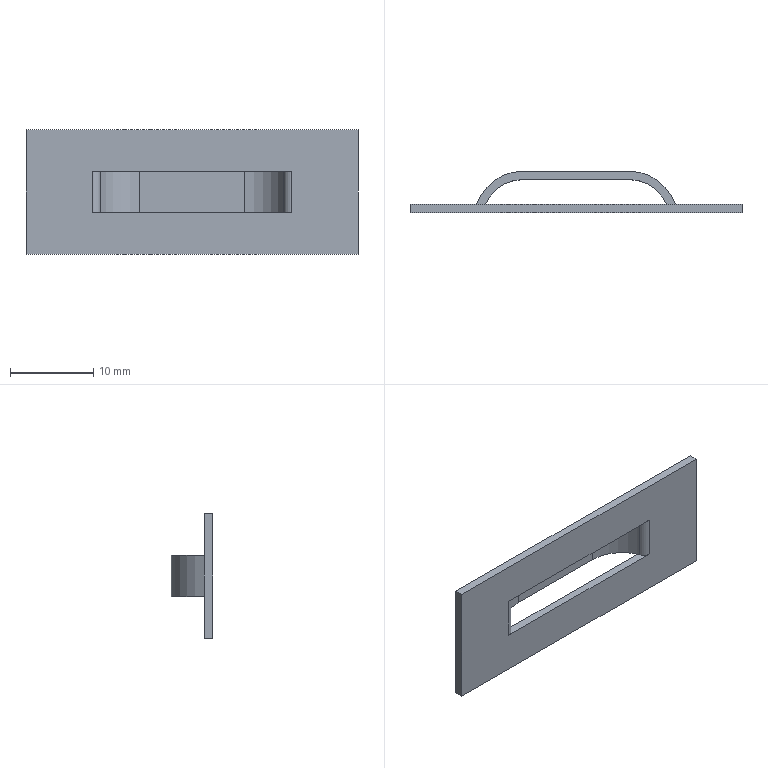Part | SolidWorks | features BaseBody 1 | 1 solid | 18 faces | box 40 x 5 x 15 mm | volume 617.289 mm3 | plane 12 | cylinder 6 | commonest cylinder face diameters 2 x2 10 x2 12 x2
STEP:
#1=CARTESIAN_POINT('',(-20.,0.,7.5));
#2=VERTEX_POINT('',#1);
#3=CARTESIAN_POINT('',(-20.,1.,7.5));
#4=VERTEX_POINT('',#3);
#5=CARTESIAN_POINT('',(-20.,-42.72,7.5));
#6=DIRECTION('',(0.,1.,0.));
#7=VECTOR('',#6,1000.);
#8=LINE('',#5,#7);
#9=EDGE_CURVE('',#2,#4,#8,.T.);
#10=ORIENTED_EDGE('',*,*,#9,.F.);
#11=CARTESIAN_POINT('',(20.,0.,7.5));
#12=VERTEX_POINT('',#11);
#13=CARTESIAN_POINT('',(20.,0.,7.5));
#14=DIRECTION('',(1.,0.,0.));
#15=VECTOR('',#14,1000.);
#16=LINE('',#13,#15);
#17=EDGE_CURVE('',#2,#12,#16,.T.);
#18=ORIENTED_EDGE('',*,*,#17,.T.);
#19=CARTESIAN_POINT('',(20.,1.,7.5));
#20=VERTEX_POINT('',#19);
#21=CARTESIAN_POINT('',(20.,-42.72,7.5));
#22=DIRECTION('',(0.,1.,0.));
#23=VECTOR('',#22,1000.);
#24=LINE('',#21,#23);
#25=EDGE_CURVE('',#12,#20,#24,.T.);
#26=ORIENTED_EDGE('',*,*,#25,.T.);
#27=CARTESIAN_POINT('',(20.,1.,7.5));
#28=DIRECTION('',(1.,0.,0.));
#29=VECTOR('',#28,1000.);
#30=LINE('',#27,#29);
#31=EDGE_CURVE('',#4,#20,#30,.T.);
#32=ORIENTED_EDGE('',*,*,#31,.F.);
#33=EDGE_LOOP('',(#10,#18,#26,#32));
#34=FACE_OUTER_BOUND('',#33,.T.);
#35=CARTESIAN_POINT('',(20.,-42.72,7.5));
#36=DIRECTION('',(0.,0.,1.));
#37=DIRECTION('',(1.,0.,0.));
#38=AXIS2_PLACEMENT_3D('',#35,#36,#37);
#39=PLANE('',#38);
#40=ADVANCED_FACE('',(#34),#39,.T.);
#41=CARTESIAN_POINT('',(-11.057,0.6667,2.5));
#42=VERTEX_POINT('',#41);
#43=CARTESIAN_POINT('',(-12.,0.,2.5));
#44=VERTEX_POINT('',#43);
#45=CARTESIAN_POINT('',(-12.,1.,2.5));
#46=DIRECTION('',(0.,0.,-1.));
#47=DIRECTION('',(1.,0.,0.));
#48=AXIS2_PLACEMENT_3D('',#45,#46,#47);
#49=CIRCLE('',#48,1.);
#50=EDGE_CURVE('',#42,#44,#49,.T.);
#51=ORIENTED_EDGE('',*,*,#50,.F.);
#52=CARTESIAN_POINT('',(-10.926,1.,2.5));
#53=VERTEX_POINT('',#52);
#54=CARTESIAN_POINT('',(-6.343,-1.,2.5));
#55=DIRECTION('',(0.,0.,1.));
#56=DIRECTION('',(-1.,0.,0.));
#57=AXIS2_PLACEMENT_3D('',#54,#55,#56);
#58=CIRCLE('',#57,5.);
#59=EDGE_CURVE('',#53,#42,#58,.T.);
#60=ORIENTED_EDGE('',*,*,#59,.F.);
#61=CARTESIAN_POINT('',(10.926,1.,2.5));
#62=VERTEX_POINT('',#61);
#63=CARTESIAN_POINT('',(12.,1.,2.5));
#64=DIRECTION('',(1.,0.,0.));
#65=VECTOR('',#64,1000.);
#66=LINE('',#63,#65);
#67=EDGE_CURVE('',#53,#62,#66,.T.);
#68=ORIENTED_EDGE('',*,*,#67,.T.);
#69=CARTESIAN_POINT('',(11.057,0.6667,2.5));
#70=VERTEX_POINT('',#69);
#71=CARTESIAN_POINT('',(6.343,-1.,2.5));
#72=DIRECTION('',(0.,0.,1.));
#73=DIRECTION('',(1.,0.,0.));
#74=AXIS2_PLACEMENT_3D('',#71,#72,#73);
#75=CIRCLE('',#74,5.);
#76=EDGE_CURVE('',#70,#62,#75,.T.);
#77=ORIENTED_EDGE('',*,*,#76,.F.);
#78=CARTESIAN_POINT('',(12.,0.,2.5));
#79=VERTEX_POINT('',#78);
#80=CARTESIAN_POINT('',(12.,1.,2.5));
#81=DIRECTION('',(0.,0.,-1.));
#82=DIRECTION('',(-1.,0.,0.));
#83=AXIS2_PLACEMENT_3D('',#80,#81,#82);
#84=CIRCLE('',#83,1.);
#85=EDGE_CURVE('',#79,#70,#84,.T.);
#86=ORIENTED_EDGE('',*,*,#85,.F.);
#87=CARTESIAN_POINT('',(12.,0.,2.5));
#88=DIRECTION('',(1.,0.,0.));
#89=VECTOR('',#88,1000.);
#90=LINE('',#87,#89);
#91=EDGE_CURVE('',#44,#79,#90,.T.);
#92=ORIENTED_EDGE('',*,*,#91,.F.);
#93=EDGE_LOOP('',(#51,#60,#68,#77,#86,#92));
#94=FACE_OUTER_BOUND('',#93,.T.);
#95=CARTESIAN_POINT('',(12.,-42.72,2.5));
#96=DIRECTION('',(0.,0.,1.));
#97=DIRECTION('',(1.,0.,0.));
#98=AXIS2_PLACEMENT_3D('',#95,#96,#97);
#99=PLANE('',#98);
#100=ADVANCED_FACE('',(#94),#99,.F.);
#101=CARTESIAN_POINT('',(-11.057,0.6667,-2.5));
#102=VERTEX_POINT('',#101);
#103=CARTESIAN_POINT('',(-12.,0.,-2.5));
#104=VERTEX_POINT('',#103);
#105=CARTESIAN_POINT('',(-12.,1.,-2.5));
#106=DIRECTION('',(0.,0.,-1.));
#107=DIRECTION('',(1.,0.,0.));
#108=AXIS2_PLACEMENT_3D('',#105,#106,#107);
#109=CIRCLE('',#108,1.);
#110=EDGE_CURVE('',#102,#104,#109,.T.);
#111=ORIENTED_EDGE('',*,*,#110,.T.);
#112=CARTESIAN_POINT('',(12.,0.,-2.5));
#113=VERTEX_POINT('',#112);
#114=CARTESIAN_POINT('',(-12.,0.,-2.5));
#115=DIRECTION('',(-1.,0.,0.));
#116=VECTOR('',#115,1000.);
#117=LINE('',#114,#116);
#118=EDGE_CURVE('',#113,#104,#117,.T.);
#119=ORIENTED_EDGE('',*,*,#118,.F.);
#120=CARTESIAN_POINT('',(11.057,0.6667,-2.5));
#121=VERTEX_POINT('',#120);
#122=CARTESIAN_POINT('',(12.,1.,-2.5));
#123=DIRECTION('',(0.,0.,-1.));
#124=DIRECTION('',(-1.,0.,0.));
#125=AXIS2_PLACEMENT_3D('',#122,#123,#124);
#126=CIRCLE('',#125,1.);
#127=EDGE_CURVE('',#113,#121,#126,.T.);
#128=ORIENTED_EDGE('',*,*,#127,.T.);
#129=CARTESIAN_POINT('',(10.926,1.,-2.5));
#130=VERTEX_POINT('',#129);
#131=CARTESIAN_POINT('',(6.343,-1.,-2.5));
#132=DIRECTION('',(0.,0.,1.));
#133=DIRECTION('',(1.,0.,0.));
#134=AXIS2_PLACEMENT_3D('',#131,#132,#133);
#135=CIRCLE('',#134,5.);
#136=EDGE_CURVE('',#121,#130,#135,.T.);
#137=ORIENTED_EDGE('',*,*,#136,.T.);
#138=CARTESIAN_POINT('',(-10.926,1.,-2.5));
#139=VERTEX_POINT('',#138);
#140=CARTESIAN_POINT('',(-12.,1.,-2.5));
#141=DIRECTION('',(-1.,0.,0.));
#142=VECTOR('',#141,1000.);
#143=LINE('',#140,#142);
#144=EDGE_CURVE('',#130,#139,#143,.T.);
#145=ORIENTED_EDGE('',*,*,#144,.T.);
#146=CARTESIAN_POINT('',(-6.343,-1.,-2.5));
#147=DIRECTION('',(0.,0.,1.));
#148=DIRECTION('',(-1.,0.,0.));
#149=AXIS2_PLACEMENT_3D('',#146,#147,#148);
#150=CIRCLE('',#149,5.);
#151=EDGE_CURVE('',#139,#102,#150,.T.);
#152=ORIENTED_EDGE('',*,*,#151,.T.);
#153=EDGE_LOOP('',(#111,#119,#128,#137,#145,#152));
#154=FACE_OUTER_BOUND('',#153,.T.);
#155=CARTESIAN_POINT('',(-12.,-42.72,-2.5));
#156=DIRECTION('',(0.,0.,-1.));
#157=DIRECTION('',(0.,-1.,0.));
#158=AXIS2_PLACEMENT_3D('',#155,#156,#157);
#159=PLANE('',#158);
#160=ADVANCED_FACE('',(#154),#159,.F.);
#161=CARTESIAN_POINT('',(20.,0.,-7.5));
#162=VERTEX_POINT('',#161);
#163=CARTESIAN_POINT('',(20.,1.,-7.5));
#164=VERTEX_POINT('',#163);
#165=CARTESIAN_POINT('',(20.,-42.72,-7.5));
#166=DIRECTION('',(0.,1.,0.));
#167=VECTOR('',#166,1000.);
#168=LINE('',#165,#167);
#169=EDGE_CURVE('',#162,#164,#168,.T.);
#170=ORIENTED_EDGE('',*,*,#169,.F.);
#171=CARTESIAN_POINT('',(-20.,0.,-7.5));
#172=VERTEX_POINT('',#171);
#173=CARTESIAN_POINT('',(20.,0.,-7.5));
#174=DIRECTION('',(-1.,0.,0.));
#175=VECTOR('',#174,1000.);
#176=LINE('',#173,#175);
#177=EDGE_CURVE('',#162,#172,#176,.T.);
#178=ORIENTED_EDGE('',*,*,#177,.T.);
#179=CARTESIAN_POINT('',(-20.,1.,-7.5));
#180=VERTEX_POINT('',#179);
#181=CARTESIAN_POINT('',(-20.,-42.72,-7.5));
#182=DIRECTION('',(0.,1.,0.));
#183=VECTOR('',#182,1000.);
#184=LINE('',#181,#183);
#185=EDGE_CURVE('',#172,#180,#184,.T.);
#186=ORIENTED_EDGE('',*,*,#185,.T.);
#187=CARTESIAN_POINT('',(20.,1.,-7.5));
#188=DIRECTION('',(-1.,0.,0.));
#189=VECTOR('',#188,1000.);
#190=LINE('',#187,#189);
#191=EDGE_CURVE('',#164,#180,#190,.T.);
#192=ORIENTED_EDGE('',*,*,#191,.F.);
#193=EDGE_LOOP('',(#170,#178,#186,#192));
#194=FACE_OUTER_BOUND('',#193,.T.);
#195=CARTESIAN_POINT('',(20.,-42.72,-7.5));
#196=DIRECTION('',(0.,0.,-1.));
#197=DIRECTION('',(0.,-1.,0.));
#198=AXIS2_PLACEMENT_3D('',#195,#196,#197);
#199=PLANE('',#198);
#200=ADVANCED_FACE('',(#194),#199,.T.);
#201=CARTESIAN_POINT('',(-6.343,5.,-2.5));
#202=VERTEX_POINT('',#201);
#203=CARTESIAN_POINT('',(-12.,1.,-2.5));
#204=VERTEX_POINT('',#203);
#205=CARTESIAN_POINT('',(-6.343,-1.,-2.5));
#206=DIRECTION('',(0.,0.,1.));
#207=DIRECTION('',(1.,0.,0.));
#208=AXIS2_PLACEMENT_3D('',#205,#206,#207);
#209=CIRCLE('',#208,6.);
#210=EDGE_CURVE('',#202,#204,#209,.T.);
#211=ORIENTED_EDGE('',*,*,#210,.T.);
#212=CARTESIAN_POINT('',(-12.,1.,2.5));
#213=VERTEX_POINT('',#212);
#214=CARTESIAN_POINT('',(-12.,1.,2.5));
#215=DIRECTION('',(0.,0.,-1.));
#216=VECTOR('',#215,1000.);
#217=LINE('',#214,#216);
#218=EDGE_CURVE('',#213,#204,#217,.T.);
#219=ORIENTED_EDGE('',*,*,#218,.F.);
#220=CARTESIAN_POINT('',(-6.343,5.,2.5));
#221=VERTEX_POINT('',#220);
#222=CARTESIAN_POINT('',(-6.343,-1.,2.5));
#223=DIRECTION('',(0.,0.,1.));
#224=DIRECTION('',(1.,0.,0.));
#225=AXIS2_PLACEMENT_3D('',#222,#223,#224);
#226=CIRCLE('',#225,6.);
#227=EDGE_CURVE('',#221,#213,#226,.T.);
#228=ORIENTED_EDGE('',*,*,#227,.F.);
#229=CARTESIAN_POINT('',(-6.343,5.,2.5));
#230=DIRECTION('',(0.,0.,-1.));
#231=VECTOR('',#230,1000.);
#232=LINE('',#229,#231);
#233=EDGE_CURVE('',#221,#202,#232,.T.);
#234=ORIENTED_EDGE('',*,*,#233,.T.);
#235=EDGE_LOOP('',(#211,#219,#228,#234));
#236=FACE_OUTER_BOUND('',#235,.T.);
#237=CARTESIAN_POINT('',(-6.343,-1.,2.5));
#238=DIRECTION('',(0.,0.,-1.));
#239=DIRECTION('',(-1.,0.,0.));
#240=AXIS2_PLACEMENT_3D('',#237,#238,#239);
#241=CYLINDRICAL_SURFACE('',#240,6.);
#242=ADVANCED_FACE('',(#236),#241,.T.);
#243=CARTESIAN_POINT('',(6.343,5.,-2.5));
#244=VERTEX_POINT('',#243);
#245=CARTESIAN_POINT('',(-6.343,5.,-2.5));
#246=DIRECTION('',(-1.,0.,0.));
#247=VECTOR('',#246,1000.);
#248=LINE('',#245,#247);
#249=EDGE_CURVE('',#244,#202,#248,.T.);
#250=ORIENTED_EDGE('',*,*,#249,.T.);
#251=ORIENTED_EDGE('',*,*,#233,.F.);
#252=CARTESIAN_POINT('',(6.343,5.,2.5));
#253=VERTEX_POINT('',#252);
#254=CARTESIAN_POINT('',(-6.343,5.,2.5));
#255=DIRECTION('',(-1.,0.,0.));
#256=VECTOR('',#255,1000.);
#257=LINE('',#254,#256);
#258=EDGE_CURVE('',#253,#221,#257,.T.);
#259=ORIENTED_EDGE('',*,*,#258,.F.);
#260=CARTESIAN_POINT('',(6.343,5.,2.5));
#261=DIRECTION('',(0.,0.,-1.));
#262=VECTOR('',#261,1000.);
#263=LINE('',#260,#262);
#264=EDGE_CURVE('',#253,#244,#263,.T.);
#265=ORIENTED_EDGE('',*,*,#264,.T.);
#266=EDGE_LOOP('',(#250,#251,#259,#265));
#267=FACE_OUTER_BOUND('',#266,.T.);
#268=CARTESIAN_POINT('',(-6.343,5.,2.5));
#269=DIRECTION('',(0.,-1.,0.));
#270=DIRECTION('',(0.,0.,-1.));
#271=AXIS2_PLACEMENT_3D('',#268,#269,#270);
#272=PLANE('',#271);
#273=ADVANCED_FACE('',(#267),#272,.F.);
#274=CARTESIAN_POINT('',(12.,1.,-2.5));
#275=VERTEX_POINT('',#274);
#276=CARTESIAN_POINT('',(6.343,-1.,-2.5));
#277=DIRECTION('',(0.,0.,1.));
#278=DIRECTION('',(1.,0.,0.));
#279=AXIS2_PLACEMENT_3D('',#276,#277,#278);
#280=CIRCLE('',#279,6.);
#281=EDGE_CURVE('',#275,#244,#280,.T.);
#282=ORIENTED_EDGE('',*,*,#281,.T.);
#283=ORIENTED_EDGE('',*,*,#264,.F.);
#284=CARTESIAN_POINT('',(12.,1.,2.5));
#285=VERTEX_POINT('',#284);
#286=CARTESIAN_POINT('',(6.343,-1.,2.5));
#287=DIRECTION('',(0.,0.,1.));
#288=DIRECTION('',(1.,0.,0.));
#289=AXIS2_PLACEMENT_3D('',#286,#287,#288);
#290=CIRCLE('',#289,6.);
#291=EDGE_CURVE('',#285,#253,#290,.T.);
#292=ORIENTED_EDGE('',*,*,#291,.F.);
#293=CARTESIAN_POINT('',(12.,1.,2.5));
#294=DIRECTION('',(0.,0.,-1.));
#295=VECTOR('',#294,1000.);
#296=LINE('',#293,#295);
#297=EDGE_CURVE('',#285,#275,#296,.T.);
#298=ORIENTED_EDGE('',*,*,#297,.T.);
#299=EDGE_LOOP('',(#282,#283,#292,#298));
#300=FACE_OUTER_BOUND('',#299,.T.);
#301=CARTESIAN_POINT('',(6.343,-1.,2.5));
#302=DIRECTION('',(0.,0.,-1.));
#303=DIRECTION('',(-1.,0.,0.));
#304=AXIS2_PLACEMENT_3D('',#301,#302,#303);
#305=CYLINDRICAL_SURFACE('',#304,6.);
#306=ADVANCED_FACE('',(#300),#305,.T.);
#307=ORIENTED_EDGE('',*,*,#297,.F.);
#308=CARTESIAN_POINT('',(12.,1.,2.5));
#309=DIRECTION('',(1.,0.,0.));
#310=VECTOR('',#309,1000.);
#311=LINE('',#308,#310);
#312=EDGE_CURVE('',#62,#285,#311,.T.);
#313=ORIENTED_EDGE('',*,*,#312,.F.);
#314=ORIENTED_EDGE('',*,*,#67,.F.);
#315=CARTESIAN_POINT('',(12.,1.,2.5));
#316=DIRECTION('',(1.,0.,0.));
#317=VECTOR('',#316,1000.);
#318=LINE('',#315,#317);
#319=EDGE_CURVE('',#213,#53,#318,.T.);
#320=ORIENTED_EDGE('',*,*,#319,.F.);
#321=ORIENTED_EDGE('',*,*,#218,.T.);
#322=CARTESIAN_POINT('',(-12.,1.,-2.5));
#323=DIRECTION('',(-1.,0.,0.));
#324=VECTOR('',#323,1000.);
#325=LINE('',#322,#324);
#326=EDGE_CURVE('',#139,#204,#325,.T.);
#327=ORIENTED_EDGE('',*,*,#326,.F.);
#328=ORIENTED_EDGE('',*,*,#144,.F.);
#329=CARTESIAN_POINT('',(-12.,1.,-2.5));
#330=DIRECTION('',(-1.,0.,0.));
#331=VECTOR('',#330,1000.);
#332=LINE('',#329,#331);
#333=EDGE_CURVE('',#275,#130,#332,.T.);
#334=ORIENTED_EDGE('',*,*,#333,.F.);
#335=EDGE_LOOP('',(#307,#313,#314,#320,#321,#327,#328,#334));
#336=FACE_BOUND('',#335,.T.);
#337=CARTESIAN_POINT('',(20.,1.,2.5));
#338=DIRECTION('',(0.,0.,-1.));
#339=VECTOR('',#338,1000.);
#340=LINE('',#337,#339);
#341=EDGE_CURVE('',#20,#164,#340,.T.);
#342=ORIENTED_EDGE('',*,*,#341,.T.);
#343=ORIENTED_EDGE('',*,*,#191,.T.);
#344=CARTESIAN_POINT('',(-20.,1.,2.5));
#345=DIRECTION('',(0.,0.,-1.));
#346=VECTOR('',#345,1000.);
#347=LINE('',#344,#346);
#348=EDGE_CURVE('',#4,#180,#347,.T.);
#349=ORIENTED_EDGE('',*,*,#348,.F.);
#350=ORIENTED_EDGE('',*,*,#31,.T.);
#351=EDGE_LOOP('',(#342,#343,#349,#350));
#352=FACE_OUTER_BOUND('',#351,.T.);
#353=CARTESIAN_POINT('',(20.,1.,2.5));
#354=DIRECTION('',(0.,-1.,0.));
#355=DIRECTION('',(-1.,0.,0.));
#356=AXIS2_PLACEMENT_3D('',#353,#354,#355);
#357=PLANE('',#356);
#358=ADVANCED_FACE('',(#336,#352),#357,.F.);
#359=CARTESIAN_POINT('',(20.,0.,2.5));
#360=DIRECTION('',(0.,0.,-1.));
#361=VECTOR('',#360,1000.);
#362=LINE('',#359,#361);
#363=EDGE_CURVE('',#12,#162,#362,.T.);
#364=ORIENTED_EDGE('',*,*,#363,.T.);
#365=ORIENTED_EDGE('',*,*,#169,.T.);
#366=ORIENTED_EDGE('',*,*,#341,.F.);
#367=ORIENTED_EDGE('',*,*,#25,.F.);
#368=EDGE_LOOP('',(#364,#365,#366,#367));
#369=FACE_OUTER_BOUND('',#368,.T.);
#370=CARTESIAN_POINT('',(20.,1.,2.5));
#371=DIRECTION('',(1.,0.,0.));
#372=DIRECTION('',(0.,1.,0.));
#373=AXIS2_PLACEMENT_3D('',#370,#371,#372);
#374=PLANE('',#373);
#375=ADVANCED_FACE('',(#369),#374,.T.);
#376=ORIENTED_EDGE('',*,*,#91,.T.);
#377=CARTESIAN_POINT('',(12.,0.,2.5));
#378=DIRECTION('',(0.,0.,-1.));
#379=VECTOR('',#378,1000.);
#380=LINE('',#377,#379);
#381=EDGE_CURVE('',#79,#113,#380,.T.);
#382=ORIENTED_EDGE('',*,*,#381,.T.);
#383=ORIENTED_EDGE('',*,*,#118,.T.);
#384=CARTESIAN_POINT('',(-12.,0.,2.5));
#385=DIRECTION('',(0.,0.,-1.));
#386=VECTOR('',#385,1000.);
#387=LINE('',#384,#386);
#388=EDGE_CURVE('',#44,#104,#387,.T.);
#389=ORIENTED_EDGE('',*,*,#388,.F.);
#390=EDGE_LOOP('',(#376,#382,#383,#389));
#391=FACE_BOUND('',#390,.T.);
#392=ORIENTED_EDGE('',*,*,#363,.F.);
#393=ORIENTED_EDGE('',*,*,#17,.F.);
#394=CARTESIAN_POINT('',(-20.,0.,2.5));
#395=DIRECTION('',(0.,0.,-1.));
#396=VECTOR('',#395,1000.);
#397=LINE('',#394,#396);
#398=EDGE_CURVE('',#2,#172,#397,.T.);
#399=ORIENTED_EDGE('',*,*,#398,.T.);
#400=ORIENTED_EDGE('',*,*,#177,.F.);
#401=EDGE_LOOP('',(#392,#393,#399,#400));
#402=FACE_OUTER_BOUND('',#401,.T.);
#403=CARTESIAN_POINT('',(20.,0.,2.5));
#404=DIRECTION('',(0.,-1.,0.));
#405=DIRECTION('',(-1.,0.,0.));
#406=AXIS2_PLACEMENT_3D('',#403,#404,#405);
#407=PLANE('',#406);
#408=ADVANCED_FACE('',(#391,#402),#407,.T.);
#409=ORIENTED_EDGE('',*,*,#127,.F.);
#410=ORIENTED_EDGE('',*,*,#381,.F.);
#411=ORIENTED_EDGE('',*,*,#85,.T.);
#412=CARTESIAN_POINT('',(11.057,0.6667,2.5));
#413=DIRECTION('',(0.,0.,-1.));
#414=VECTOR('',#413,1000.);
#415=LINE('',#412,#414);
#416=EDGE_CURVE('',#70,#121,#415,.T.);
#417=ORIENTED_EDGE('',*,*,#416,.T.);
#418=EDGE_LOOP('',(#409,#410,#411,#417));
#419=FACE_OUTER_BOUND('',#418,.T.);
#420=CARTESIAN_POINT('',(12.,1.,2.5));
#421=DIRECTION('',(0.,0.,-1.));
#422=DIRECTION('',(-1.,0.,0.));
#423=AXIS2_PLACEMENT_3D('',#420,#421,#422);
#424=CYLINDRICAL_SURFACE('',#423,1.);
#425=ADVANCED_FACE('',(#419),#424,.T.);
#426=ORIENTED_EDGE('',*,*,#136,.F.);
#427=ORIENTED_EDGE('',*,*,#416,.F.);
#428=ORIENTED_EDGE('',*,*,#76,.T.);
#429=CARTESIAN_POINT('',(6.343,4.,2.5));
#430=VERTEX_POINT('',#429);
#431=CARTESIAN_POINT('',(6.343,-1.,2.5));
#432=DIRECTION('',(0.,0.,1.));
#433=DIRECTION('',(1.,0.,0.));
#434=AXIS2_PLACEMENT_3D('',#431,#432,#433);
#435=CIRCLE('',#434,5.);
#436=EDGE_CURVE('',#62,#430,#435,.T.);
#437=ORIENTED_EDGE('',*,*,#436,.T.);
#438=CARTESIAN_POINT('',(6.343,4.,-2.5));
#439=VERTEX_POINT('',#438);
#440=CARTESIAN_POINT('',(6.343,4.,2.5));
#441=DIRECTION('',(0.,0.,-1.));
#442=VECTOR('',#441,1000.);
#443=LINE('',#440,#442);
#444=EDGE_CURVE('',#430,#439,#443,.T.);
#445=ORIENTED_EDGE('',*,*,#444,.T.);
#446=CARTESIAN_POINT('',(6.343,-1.,-2.5));
#447=DIRECTION('',(0.,0.,1.));
#448=DIRECTION('',(1.,0.,0.));
#449=AXIS2_PLACEMENT_3D('',#446,#447,#448);
#450=CIRCLE('',#449,5.);
#451=EDGE_CURVE('',#130,#439,#450,.T.);
#452=ORIENTED_EDGE('',*,*,#451,.F.);
#453=EDGE_LOOP('',(#426,#427,#428,#437,#445,#452));
#454=FACE_OUTER_BOUND('',#453,.T.);
#455=CARTESIAN_POINT('',(6.343,-1.,2.5));
#456=DIRECTION('',(0.,0.,-1.));
#457=DIRECTION('',(-1.,0.,0.));
#458=AXIS2_PLACEMENT_3D('',#455,#456,#457);
#459=CYLINDRICAL_SURFACE('',#458,5.);
#460=ADVANCED_FACE('',(#454),#459,.F.);
#461=CARTESIAN_POINT('',(-6.343,4.,-2.5));
#462=VERTEX_POINT('',#461);
#463=CARTESIAN_POINT('',(-6.343,4.,-2.5));
#464=DIRECTION('',(-1.,0.,0.));
#465=VECTOR('',#464,1000.);
#466=LINE('',#463,#465);
#467=EDGE_CURVE('',#439,#462,#466,.T.);
#468=ORIENTED_EDGE('',*,*,#467,.F.);
#469=ORIENTED_EDGE('',*,*,#444,.F.);
#470=CARTESIAN_POINT('',(-6.343,4.,2.5));
#471=VERTEX_POINT('',#470);
#472=CARTESIAN_POINT('',(-6.343,4.,2.5));
#473=DIRECTION('',(-1.,0.,0.));
#474=VECTOR('',#473,1000.);
#475=LINE('',#472,#474);
#476=EDGE_CURVE('',#430,#471,#475,.T.);
#477=ORIENTED_EDGE('',*,*,#476,.T.);
#478=CARTESIAN_POINT('',(-6.343,4.,2.5));
#479=DIRECTION('',(0.,0.,-1.));
#480=VECTOR('',#479,1000.);
#481=LINE('',#478,#480);
#482=EDGE_CURVE('',#471,#462,#481,.T.);
#483=ORIENTED_EDGE('',*,*,#482,.T.);
#484=EDGE_LOOP('',(#468,#469,#477,#483));
#485=FACE_OUTER_BOUND('',#484,.T.);
#486=CARTESIAN_POINT('',(-6.343,4.,2.5));
#487=DIRECTION('',(0.,-1.,0.));
#488=DIRECTION('',(0.,0.,-1.));
#489=AXIS2_PLACEMENT_3D('',#486,#487,#488);
#490=PLANE('',#489);
#491=ADVANCED_FACE('',(#485),#490,.T.);
#492=CARTESIAN_POINT('',(-6.343,-1.,-2.5));
#493=DIRECTION('',(0.,0.,1.));
#494=DIRECTION('',(-1.,0.,0.));
#495=AXIS2_PLACEMENT_3D('',#492,#493,#494);
#496=CIRCLE('',#495,5.);
#497=EDGE_CURVE('',#462,#139,#496,.T.);
#498=ORIENTED_EDGE('',*,*,#497,.F.);
#499=ORIENTED_EDGE('',*,*,#482,.F.);
#500=CARTESIAN_POINT('',(-6.343,-1.,2.5));
#501=DIRECTION('',(0.,0.,1.));
#502=DIRECTION('',(-1.,0.,0.));
#503=AXIS2_PLACEMENT_3D('',#500,#501,#502);
#504=CIRCLE('',#503,5.);
#505=EDGE_CURVE('',#471,#53,#504,.T.);
#506=ORIENTED_EDGE('',*,*,#505,.T.);
#507=ORIENTED_EDGE('',*,*,#59,.T.);
#508=CARTESIAN_POINT('',(-11.057,0.6667,2.5));
#509=DIRECTION('',(0.,0.,-1.));
#510=VECTOR('',#509,1000.);
#511=LINE('',#508,#510);
#512=EDGE_CURVE('',#42,#102,#511,.T.);
#513=ORIENTED_EDGE('',*,*,#512,.T.);
#514=ORIENTED_EDGE('',*,*,#151,.F.);
#515=EDGE_LOOP('',(#498,#499,#506,#507,#513,#514));
#516=FACE_OUTER_BOUND('',#515,.T.);
#517=CARTESIAN_POINT('',(-6.343,-1.,2.5));
#518=DIRECTION('',(0.,0.,-1.));
#519=DIRECTION('',(-1.,0.,0.));
#520=AXIS2_PLACEMENT_3D('',#517,#518,#519);
#521=CYLINDRICAL_SURFACE('',#520,5.);
#522=ADVANCED_FACE('',(#516),#521,.F.);
#523=ORIENTED_EDGE('',*,*,#110,.F.);
#524=ORIENTED_EDGE('',*,*,#512,.F.);
#525=ORIENTED_EDGE('',*,*,#50,.T.);
#526=ORIENTED_EDGE('',*,*,#388,.T.);
#527=EDGE_LOOP('',(#523,#524,#525,#526));
#528=FACE_OUTER_BOUND('',#527,.T.);
#529=CARTESIAN_POINT('',(-12.,1.,2.5));
#530=DIRECTION('',(0.,0.,-1.));
#531=DIRECTION('',(-1.,0.,0.));
#532=AXIS2_PLACEMENT_3D('',#529,#530,#531);
#533=CYLINDRICAL_SURFACE('',#532,1.);
#534=ADVANCED_FACE('',(#528),#533,.T.);
#535=ORIENTED_EDGE('',*,*,#348,.T.);
#536=ORIENTED_EDGE('',*,*,#185,.F.);
#537=ORIENTED_EDGE('',*,*,#398,.F.);
#538=ORIENTED_EDGE('',*,*,#9,.T.);
#539=EDGE_LOOP('',(#535,#536,#537,#538));
#540=FACE_OUTER_BOUND('',#539,.T.);
#541=CARTESIAN_POINT('',(-20.,0.,2.5));
#542=DIRECTION('',(-1.,0.,0.));
#543=DIRECTION('',(0.,0.,1.));
#544=AXIS2_PLACEMENT_3D('',#541,#542,#543);
#545=PLANE('',#544);
#546=ADVANCED_FACE('',(#540),#545,.T.);
#547=ORIENTED_EDGE('',*,*,#281,.F.);
#548=ORIENTED_EDGE('',*,*,#333,.T.);
#549=ORIENTED_EDGE('',*,*,#451,.T.);
#550=ORIENTED_EDGE('',*,*,#467,.T.);
#551=ORIENTED_EDGE('',*,*,#497,.T.);
#552=ORIENTED_EDGE('',*,*,#326,.T.);
#553=ORIENTED_EDGE('',*,*,#210,.F.);
#554=ORIENTED_EDGE('',*,*,#249,.F.);
#555=EDGE_LOOP('',(#547,#548,#549,#550,#551,#552,#553,#554));
#556=FACE_OUTER_BOUND('',#555,.T.);
#557=CARTESIAN_POINT('',(-12.,1.,-2.5));
#558=DIRECTION('',(0.,0.,-1.));
#559=DIRECTION('',(0.,-1.,0.));
#560=AXIS2_PLACEMENT_3D('',#557,#558,#559);
#561=PLANE('',#560);
#562=ADVANCED_FACE('',(#556),#561,.T.);
#563=ORIENTED_EDGE('',*,*,#312,.T.);
#564=ORIENTED_EDGE('',*,*,#291,.T.);
#565=ORIENTED_EDGE('',*,*,#258,.T.);
#566=ORIENTED_EDGE('',*,*,#227,.T.);
#567=ORIENTED_EDGE('',*,*,#319,.T.);
#568=ORIENTED_EDGE('',*,*,#505,.F.);
#569=ORIENTED_EDGE('',*,*,#476,.F.);
#570=ORIENTED_EDGE('',*,*,#436,.F.);
#571=EDGE_LOOP('',(#563,#564,#565,#566,#567,#568,#569,#570));
#572=FACE_OUTER_BOUND('',#571,.T.);
#573=CARTESIAN_POINT('',(-12.,1.,2.5));
#574=DIRECTION('',(0.,0.,-1.));
#575=DIRECTION('',(0.,-1.,0.));
#576=AXIS2_PLACEMENT_3D('',#573,#574,#575);
#577=PLANE('',#576);
#578=ADVANCED_FACE('',(#572),#577,.F.);
#579=CLOSED_SHELL('',(#40,#100,#160,#200,#242,#273,#306,#358,#375,#408,#425,#460,#491,#522,#534,#546,#562,#578));
#580=MANIFOLD_SOLID_BREP('',#579);
#581=CARTESIAN_POINT('',(0.,0.,0.));
#582=DIRECTION('',(0.,0.,1.));
#583=DIRECTION('',(1.,0.,0.));
#584=AXIS2_PLACEMENT_3D('',#581,#582,#583);
#585=(LENGTH_UNIT()NAMED_UNIT(*)SI_UNIT(.MILLI.,.METRE.));
#586=UNCERTAINTY_MEASURE_WITH_UNIT(LENGTH_MEASURE(0.00001),#585,'','');
#587=(NAMED_UNIT(*)PLANE_ANGLE_UNIT()SI_UNIT($,.RADIAN.));
#588=(NAMED_UNIT(*)SI_UNIT($,.STERADIAN.)SOLID_ANGLE_UNIT());
#589=(GEOMETRIC_REPRESENTATION_CONTEXT(3)GLOBAL_UNCERTAINTY_ASSIGNED_CONTEXT((#586))GLOBAL_UNIT_ASSIGNED_CONTEXT((#585,#587,#588))REPRESENTATION_CONTEXT('',''));
#590=ADVANCED_BREP_SHAPE_REPRESENTATION('',(#580,#584),#589);